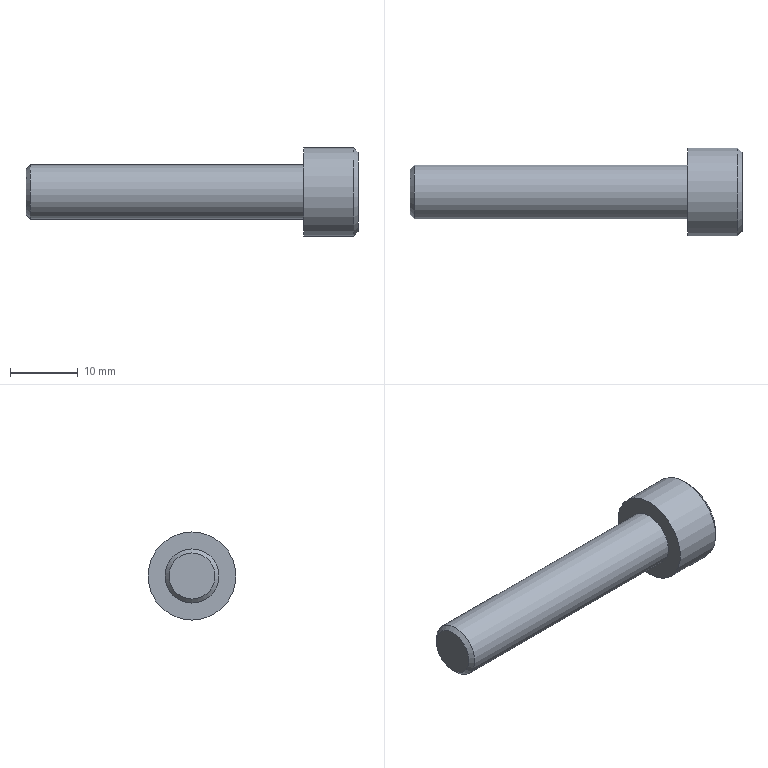Part | NX | features M8.00-60.00 2 | 1 solid | 14 faces | box 49 x 13 x 13 mm | volume 2951 mm3 | plane 10 | cylinder 2 | cone 2 | commonest cylinder face diameters 8 x1 13 x1
STEP:
#1=CARTESIAN_POINT('',(113.275,-14.,-17.451));
#2=VERTEX_POINT('',#1);
#3=CARTESIAN_POINT('',(113.275,-14.,-11.551));
#4=DIRECTION('',(1.,0.,0.));
#5=DIRECTION('',(0.,0.,-1.));
#6=AXIS2_PLACEMENT_3D('',#3,#4,#5);
#7=CIRCLE('',#6,5.9);
#8=EDGE_CURVE('',#2,#2,#7,.T.);
#9=ORIENTED_EDGE('',*,*,#8,.T.);
#10=EDGE_LOOP('',(#9));
#11=FACE_BOUND('',#10,.T.);
#12=CARTESIAN_POINT('',(113.275,-17.4,-9.588));
#13=VERTEX_POINT('',#12);
#14=CARTESIAN_POINT('',(113.275,-17.4,-13.514));
#15=VERTEX_POINT('',#14);
#16=CARTESIAN_POINT('',(113.275,-17.4,-9.588));
#17=DIRECTION('',(0.,0.,-1.));
#18=VECTOR('',#17,1000.);
#19=LINE('',#16,#18);
#20=EDGE_CURVE('',#13,#15,#19,.T.);
#21=ORIENTED_EDGE('',*,*,#20,.F.);
#22=CARTESIAN_POINT('',(113.275,-14.,-7.625));
#23=VERTEX_POINT('',#22);
#24=CARTESIAN_POINT('',(113.275,-14.,-7.625));
#25=DIRECTION('',(0.,-0.866,-0.5));
#26=VECTOR('',#25,1000.);
#27=LINE('',#24,#26);
#28=EDGE_CURVE('',#23,#13,#27,.T.);
#29=ORIENTED_EDGE('',*,*,#28,.F.);
#30=CARTESIAN_POINT('',(113.275,-10.6,-9.588));
#31=VERTEX_POINT('',#30);
#32=CARTESIAN_POINT('',(113.275,-10.6,-9.588));
#33=DIRECTION('',(0.,-0.866,0.5));
#34=VECTOR('',#33,1000.);
#35=LINE('',#32,#34);
#36=EDGE_CURVE('',#31,#23,#35,.T.);
#37=ORIENTED_EDGE('',*,*,#36,.F.);
#38=CARTESIAN_POINT('',(113.275,-10.6,-13.514));
#39=VERTEX_POINT('',#38);
#40=CARTESIAN_POINT('',(113.275,-10.6,-13.514));
#41=DIRECTION('',(0.,0.,1.));
#42=VECTOR('',#41,1000.);
#43=LINE('',#40,#42);
#44=EDGE_CURVE('',#39,#31,#43,.T.);
#45=ORIENTED_EDGE('',*,*,#44,.F.);
#46=CARTESIAN_POINT('',(113.275,-14.,-15.477));
#47=VERTEX_POINT('',#46);
#48=CARTESIAN_POINT('',(113.275,-14.,-15.477));
#49=DIRECTION('',(0.,0.866,0.5));
#50=VECTOR('',#49,1000.);
#51=LINE('',#48,#50);
#52=EDGE_CURVE('',#47,#39,#51,.T.);
#53=ORIENTED_EDGE('',*,*,#52,.F.);
#54=CARTESIAN_POINT('',(113.275,-17.4,-13.514));
#55=DIRECTION('',(0.,0.866,-0.5));
#56=VECTOR('',#55,1000.);
#57=LINE('',#54,#56);
#58=EDGE_CURVE('',#15,#47,#57,.T.);
#59=ORIENTED_EDGE('',*,*,#58,.F.);
#60=EDGE_LOOP('',(#21,#29,#37,#45,#53,#59));
#61=FACE_BOUND('',#60,.T.);
#62=CARTESIAN_POINT('',(113.275,-14.,-11.551));
#63=DIRECTION('',(1.,0.,0.));
#64=DIRECTION('',(0.,0.,-1.));
#65=AXIS2_PLACEMENT_3D('',#62,#63,#64);
#66=PLANE('',#65);
#67=ADVANCED_FACE('',(#11,#61),#66,.T.);
#68=CARTESIAN_POINT('',(105.275,-14.,-7.551));
#69=VERTEX_POINT('',#68);
#70=CARTESIAN_POINT('',(105.275,-14.,-11.551));
#71=DIRECTION('',(-1.,0.,0.));
#72=DIRECTION('',(0.,0.,1.));
#73=AXIS2_PLACEMENT_3D('',#70,#71,#72);
#74=CIRCLE('',#73,4.);
#75=EDGE_CURVE('',#69,#69,#74,.T.);
#76=ORIENTED_EDGE('',*,*,#75,.F.);
#77=EDGE_LOOP('',(#76));
#78=FACE_BOUND('',#77,.T.);
#79=CARTESIAN_POINT('',(105.275,-14.,-18.051));
#80=VERTEX_POINT('',#79);
#81=CARTESIAN_POINT('',(105.275,-14.,-11.551));
#82=DIRECTION('',(1.,0.,0.));
#83=DIRECTION('',(0.,0.,-1.));
#84=AXIS2_PLACEMENT_3D('',#81,#82,#83);
#85=CIRCLE('',#84,6.5);
#86=EDGE_CURVE('',#80,#80,#85,.T.);
#87=ORIENTED_EDGE('',*,*,#86,.F.);
#88=EDGE_LOOP('',(#87));
#89=FACE_BOUND('',#88,.T.);
#90=CARTESIAN_POINT('',(105.275,-14.,-11.551));
#91=DIRECTION('',(-1.,0.,0.));
#92=DIRECTION('',(0.,0.,1.));
#93=AXIS2_PLACEMENT_3D('',#90,#91,#92);
#94=PLANE('',#93);
#95=ADVANCED_FACE('',(#78,#89),#94,.T.);
#96=CARTESIAN_POINT('',(112.675,-14.,-18.051));
#97=VERTEX_POINT('',#96);
#98=CARTESIAN_POINT('',(112.675,-14.,-11.551));
#99=DIRECTION('',(1.,0.,0.));
#100=DIRECTION('',(0.,0.,-1.));
#101=AXIS2_PLACEMENT_3D('',#98,#99,#100);
#102=CIRCLE('',#101,6.5);
#103=EDGE_CURVE('',#97,#97,#102,.F.);
#104=ORIENTED_EDGE('',*,*,#103,.T.);
#105=EDGE_LOOP('',(#104));
#106=FACE_BOUND('',#105,.T.);
#107=ORIENTED_EDGE('',*,*,#86,.T.);
#108=EDGE_LOOP('',(#107));
#109=FACE_BOUND('',#108,.T.);
#110=CARTESIAN_POINT('',(105.275,-14.,-11.551));
#111=DIRECTION('',(1.,0.,0.));
#112=DIRECTION('',(0.,0.,-1.));
#113=AXIS2_PLACEMENT_3D('',#110,#111,#112);
#114=CYLINDRICAL_SURFACE('',#113,6.5);
#115=ADVANCED_FACE('',(#106,#109),#114,.T.);
#116=CARTESIAN_POINT('',(64.275,-14.,-8.151));
#117=VERTEX_POINT('',#116);
#118=CARTESIAN_POINT('',(64.275,-14.,-11.551));
#119=DIRECTION('',(-1.,0.,0.));
#120=DIRECTION('',(0.,0.,1.));
#121=AXIS2_PLACEMENT_3D('',#118,#119,#120);
#122=CIRCLE('',#121,3.4);
#123=EDGE_CURVE('',#117,#117,#122,.T.);
#124=ORIENTED_EDGE('',*,*,#123,.T.);
#125=EDGE_LOOP('',(#124));
#126=FACE_BOUND('',#125,.T.);
#127=CARTESIAN_POINT('',(64.275,-14.,-11.551));
#128=DIRECTION('',(-1.,0.,0.));
#129=DIRECTION('',(0.,0.,1.));
#130=AXIS2_PLACEMENT_3D('',#127,#128,#129);
#131=PLANE('',#130);
#132=ADVANCED_FACE('',(#126),#131,.T.);
#133=CARTESIAN_POINT('',(64.875,-14.,-7.551));
#134=VERTEX_POINT('',#133);
#135=CARTESIAN_POINT('',(64.875,-14.,-11.551));
#136=DIRECTION('',(-1.,0.,0.));
#137=DIRECTION('',(0.,0.,1.));
#138=AXIS2_PLACEMENT_3D('',#135,#136,#137);
#139=CIRCLE('',#138,4.);
#140=EDGE_CURVE('',#134,#134,#139,.F.);
#141=ORIENTED_EDGE('',*,*,#140,.T.);
#142=EDGE_LOOP('',(#141));
#143=FACE_BOUND('',#142,.T.);
#144=ORIENTED_EDGE('',*,*,#75,.T.);
#145=EDGE_LOOP('',(#144));
#146=FACE_BOUND('',#145,.T.);
#147=CARTESIAN_POINT('',(116.275,-14.,-11.551));
#148=DIRECTION('',(-1.,0.,0.));
#149=DIRECTION('',(0.,0.,1.));
#150=AXIS2_PLACEMENT_3D('',#147,#148,#149);
#151=CYLINDRICAL_SURFACE('',#150,4.);
#152=ADVANCED_FACE('',(#143,#146),#151,.T.);
#153=ORIENTED_EDGE('',*,*,#58,.T.);
#154=CARTESIAN_POINT('',(109.275,-14.,-15.477));
#155=VERTEX_POINT('',#154);
#156=CARTESIAN_POINT('',(109.275,-14.,-15.477));
#157=DIRECTION('',(1.,0.,0.));
#158=VECTOR('',#157,1000.);
#159=LINE('',#156,#158);
#160=EDGE_CURVE('',#47,#155,#159,.F.);
#161=ORIENTED_EDGE('',*,*,#160,.T.);
#162=CARTESIAN_POINT('',(109.275,-17.4,-13.514));
#163=VERTEX_POINT('',#162);
#164=CARTESIAN_POINT('',(109.275,-17.4,-13.514));
#165=DIRECTION('',(0.,0.866,-0.5));
#166=VECTOR('',#165,1000.);
#167=LINE('',#164,#166);
#168=EDGE_CURVE('',#155,#163,#167,.F.);
#169=ORIENTED_EDGE('',*,*,#168,.T.);
#170=CARTESIAN_POINT('',(109.275,-17.4,-13.514));
#171=DIRECTION('',(1.,0.,0.));
#172=VECTOR('',#171,1000.);
#173=LINE('',#170,#172);
#174=EDGE_CURVE('',#15,#163,#173,.F.);
#175=ORIENTED_EDGE('',*,*,#174,.F.);
#176=EDGE_LOOP('',(#153,#161,#169,#175));
#177=FACE_BOUND('',#176,.T.);
#178=CARTESIAN_POINT('',(111.275,-15.7,-14.496));
#179=DIRECTION('',(0.,-0.5,-0.866));
#180=DIRECTION('',(0.,0.866,-0.5));
#181=AXIS2_PLACEMENT_3D('',#178,#179,#180);
#182=PLANE('',#181);
#183=ADVANCED_FACE('',(#177),#182,.F.);
#184=ORIENTED_EDGE('',*,*,#20,.T.);
#185=ORIENTED_EDGE('',*,*,#174,.T.);
#186=CARTESIAN_POINT('',(109.275,-17.4,-9.588));
#187=VERTEX_POINT('',#186);
#188=CARTESIAN_POINT('',(109.275,-17.4,-9.588));
#189=DIRECTION('',(0.,0.,-1.));
#190=VECTOR('',#189,1000.);
#191=LINE('',#188,#190);
#192=EDGE_CURVE('',#163,#187,#191,.F.);
#193=ORIENTED_EDGE('',*,*,#192,.T.);
#194=CARTESIAN_POINT('',(109.275,-17.4,-9.588));
#195=DIRECTION('',(1.,0.,0.));
#196=VECTOR('',#195,1000.);
#197=LINE('',#194,#196);
#198=EDGE_CURVE('',#13,#187,#197,.F.);
#199=ORIENTED_EDGE('',*,*,#198,.F.);
#200=EDGE_LOOP('',(#184,#185,#193,#199));
#201=FACE_BOUND('',#200,.T.);
#202=CARTESIAN_POINT('',(111.275,-17.4,-11.551));
#203=DIRECTION('',(0.,-1.,0.));
#204=DIRECTION('',(1.,0.,0.));
#205=AXIS2_PLACEMENT_3D('',#202,#203,#204);
#206=PLANE('',#205);
#207=ADVANCED_FACE('',(#201),#206,.F.);
#208=ORIENTED_EDGE('',*,*,#28,.T.);
#209=ORIENTED_EDGE('',*,*,#198,.T.);
#210=CARTESIAN_POINT('',(109.275,-14.,-7.625));
#211=VERTEX_POINT('',#210);
#212=CARTESIAN_POINT('',(109.275,-14.,-7.625));
#213=DIRECTION('',(0.,-0.866,-0.5));
#214=VECTOR('',#213,1000.);
#215=LINE('',#212,#214);
#216=EDGE_CURVE('',#187,#211,#215,.F.);
#217=ORIENTED_EDGE('',*,*,#216,.T.);
#218=CARTESIAN_POINT('',(109.275,-14.,-7.625));
#219=DIRECTION('',(1.,0.,0.));
#220=VECTOR('',#219,1000.);
#221=LINE('',#218,#220);
#222=EDGE_CURVE('',#23,#211,#221,.F.);
#223=ORIENTED_EDGE('',*,*,#222,.F.);
#224=EDGE_LOOP('',(#208,#209,#217,#223));
#225=FACE_BOUND('',#224,.T.);
#226=CARTESIAN_POINT('',(111.275,-15.7,-8.607));
#227=DIRECTION('',(0.,-0.5,0.866));
#228=DIRECTION('',(0.,-0.866,-0.5));
#229=AXIS2_PLACEMENT_3D('',#226,#227,#228);
#230=PLANE('',#229);
#231=ADVANCED_FACE('',(#225),#230,.F.);
#232=ORIENTED_EDGE('',*,*,#36,.T.);
#233=ORIENTED_EDGE('',*,*,#222,.T.);
#234=CARTESIAN_POINT('',(109.275,-10.6,-9.588));
#235=VERTEX_POINT('',#234);
#236=CARTESIAN_POINT('',(109.275,-10.6,-9.588));
#237=DIRECTION('',(0.,-0.866,0.5));
#238=VECTOR('',#237,1000.);
#239=LINE('',#236,#238);
#240=EDGE_CURVE('',#211,#235,#239,.F.);
#241=ORIENTED_EDGE('',*,*,#240,.T.);
#242=CARTESIAN_POINT('',(109.275,-10.6,-9.588));
#243=DIRECTION('',(1.,0.,0.));
#244=VECTOR('',#243,1000.);
#245=LINE('',#242,#244);
#246=EDGE_CURVE('',#31,#235,#245,.F.);
#247=ORIENTED_EDGE('',*,*,#246,.F.);
#248=EDGE_LOOP('',(#232,#233,#241,#247));
#249=FACE_BOUND('',#248,.T.);
#250=CARTESIAN_POINT('',(111.275,-12.3,-8.607));
#251=DIRECTION('',(0.,0.5,0.866));
#252=DIRECTION('',(0.,-0.866,0.5));
#253=AXIS2_PLACEMENT_3D('',#250,#251,#252);
#254=PLANE('',#253);
#255=ADVANCED_FACE('',(#249),#254,.F.);
#256=ORIENTED_EDGE('',*,*,#44,.T.);
#257=ORIENTED_EDGE('',*,*,#246,.T.);
#258=CARTESIAN_POINT('',(109.275,-10.6,-13.514));
#259=VERTEX_POINT('',#258);
#260=CARTESIAN_POINT('',(109.275,-10.6,-13.514));
#261=DIRECTION('',(0.,0.,1.));
#262=VECTOR('',#261,1000.);
#263=LINE('',#260,#262);
#264=EDGE_CURVE('',#235,#259,#263,.F.);
#265=ORIENTED_EDGE('',*,*,#264,.T.);
#266=CARTESIAN_POINT('',(109.275,-10.6,-13.514));
#267=DIRECTION('',(1.,0.,0.));
#268=VECTOR('',#267,1000.);
#269=LINE('',#266,#268);
#270=EDGE_CURVE('',#39,#259,#269,.F.);
#271=ORIENTED_EDGE('',*,*,#270,.F.);
#272=EDGE_LOOP('',(#256,#257,#265,#271));
#273=FACE_BOUND('',#272,.T.);
#274=CARTESIAN_POINT('',(111.275,-10.6,-11.551));
#275=DIRECTION('',(0.,1.,0.));
#276=DIRECTION('',(-1.,0.,0.));
#277=AXIS2_PLACEMENT_3D('',#274,#275,#276);
#278=PLANE('',#277);
#279=ADVANCED_FACE('',(#273),#278,.F.);
#280=ORIENTED_EDGE('',*,*,#52,.T.);
#281=ORIENTED_EDGE('',*,*,#270,.T.);
#282=CARTESIAN_POINT('',(109.275,-14.,-15.477));
#283=DIRECTION('',(0.,0.866,0.5));
#284=VECTOR('',#283,1000.);
#285=LINE('',#282,#284);
#286=EDGE_CURVE('',#259,#155,#285,.F.);
#287=ORIENTED_EDGE('',*,*,#286,.T.);
#288=ORIENTED_EDGE('',*,*,#160,.F.);
#289=EDGE_LOOP('',(#280,#281,#287,#288));
#290=FACE_BOUND('',#289,.T.);
#291=CARTESIAN_POINT('',(111.275,-12.3,-14.496));
#292=DIRECTION('',(0.,0.5,-0.866));
#293=DIRECTION('',(0.,0.866,0.5));
#294=AXIS2_PLACEMENT_3D('',#291,#292,#293);
#295=PLANE('',#294);
#296=ADVANCED_FACE('',(#290),#295,.F.);
#297=ORIENTED_EDGE('',*,*,#286,.F.);
#298=ORIENTED_EDGE('',*,*,#264,.F.);
#299=ORIENTED_EDGE('',*,*,#240,.F.);
#300=ORIENTED_EDGE('',*,*,#216,.F.);
#301=ORIENTED_EDGE('',*,*,#192,.F.);
#302=ORIENTED_EDGE('',*,*,#168,.F.);
#303=EDGE_LOOP('',(#297,#298,#299,#300,#301,#302));
#304=FACE_BOUND('',#303,.T.);
#305=CARTESIAN_POINT('',(109.275,-14.,-11.551));
#306=DIRECTION('',(-1.,0.,0.));
#307=DIRECTION('',(0.,0.,1.));
#308=AXIS2_PLACEMENT_3D('',#305,#306,#307);
#309=PLANE('',#308);
#310=ADVANCED_FACE('',(#304),#309,.F.);
#311=ORIENTED_EDGE('',*,*,#123,.F.);
#312=EDGE_LOOP('',(#311));
#313=FACE_BOUND('',#312,.T.);
#314=ORIENTED_EDGE('',*,*,#140,.F.);
#315=EDGE_LOOP('',(#314));
#316=FACE_BOUND('',#315,.T.);
#317=CARTESIAN_POINT('',(64.875,-14.,-11.551));
#318=DIRECTION('',(1.,0.,0.));
#319=DIRECTION('',(0.,0.,-1.));
#320=AXIS2_PLACEMENT_3D('',#317,#318,#319);
#321=CONICAL_SURFACE('',#320,4.,0.7854);
#322=ADVANCED_FACE('',(#313,#316),#321,.T.);
#323=ORIENTED_EDGE('',*,*,#8,.F.);
#324=EDGE_LOOP('',(#323));
#325=FACE_BOUND('',#324,.T.);
#326=ORIENTED_EDGE('',*,*,#103,.F.);
#327=EDGE_LOOP('',(#326));
#328=FACE_BOUND('',#327,.T.);
#329=CARTESIAN_POINT('',(112.675,-14.,-11.551));
#330=DIRECTION('',(-1.,0.,0.));
#331=DIRECTION('',(0.,0.,1.));
#332=AXIS2_PLACEMENT_3D('',#329,#330,#331);
#333=CONICAL_SURFACE('',#332,6.5,0.7854);
#334=ADVANCED_FACE('',(#325,#328),#333,.T.);
#335=CLOSED_SHELL('',(#67,#95,#115,#132,#152,#183,#207,#231,#255,#279,#296,#310,#322,#334));
#336=MANIFOLD_SOLID_BREP('',#335);
#337=(LENGTH_UNIT()NAMED_UNIT(*)SI_UNIT(.MILLI.,.METRE.));
#338=UNCERTAINTY_MEASURE_WITH_UNIT(LENGTH_MEASURE(0.00001),#337,'','');
#339=(NAMED_UNIT(*)PLANE_ANGLE_UNIT()SI_UNIT($,.RADIAN.));
#340=(NAMED_UNIT(*)SI_UNIT($,.STERADIAN.)SOLID_ANGLE_UNIT());
#341=(GEOMETRIC_REPRESENTATION_CONTEXT(3)GLOBAL_UNCERTAINTY_ASSIGNED_CONTEXT((#338))GLOBAL_UNIT_ASSIGNED_CONTEXT((#337,#339,#340))REPRESENTATION_CONTEXT('',''));
#342=ADVANCED_BREP_SHAPE_REPRESENTATION('',(#336),#341);